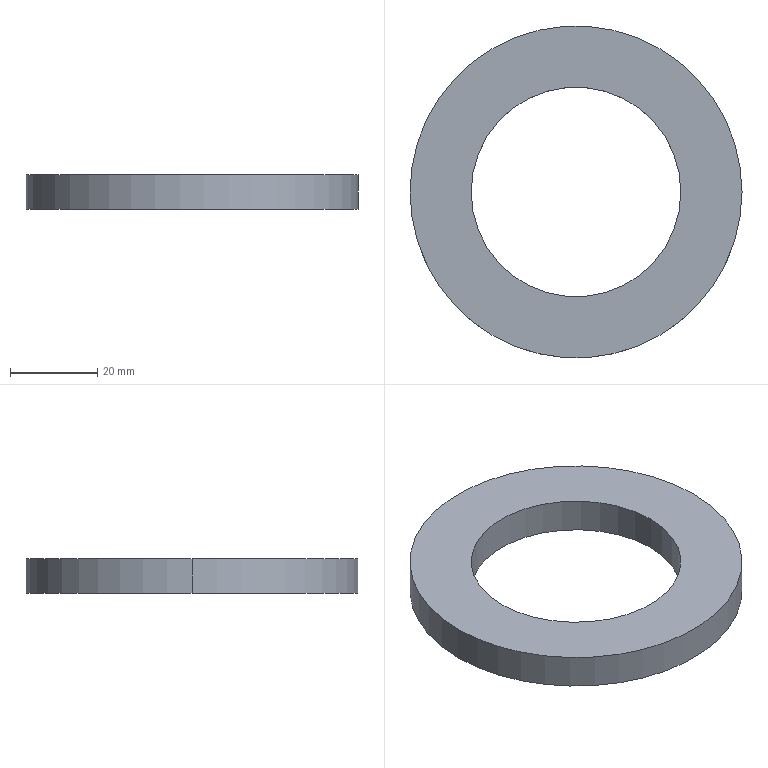Part | SolidWorks | features Extrusion 1 | 1 solid | 6 faces | box 76 x 76 x 8 mm | volume 21815 mm3 | cylinder 4 | plane 2 | commonest cylinder face diameters 48 x2 76 x2
STEP:
#1=CARTESIAN_POINT('',(-24.,0.,8.));
#2=VERTEX_POINT('',#1);
#3=CARTESIAN_POINT('',(24.,0.,8.));
#4=VERTEX_POINT('',#3);
#5=CARTESIAN_POINT('',(0.,0.,8.));
#6=DIRECTION('',(0.,0.,1.));
#7=DIRECTION('',(1.,0.,0.));
#8=AXIS2_PLACEMENT_3D('',#5,#6,#7);
#9=CIRCLE('',#8,24.);
#10=EDGE_CURVE('',#2,#4,#9,.T.);
#11=ORIENTED_EDGE('',*,*,#10,.T.);
#12=CARTESIAN_POINT('',(24.,0.,0.));
#13=VERTEX_POINT('',#12);
#14=CARTESIAN_POINT('',(24.,0.,8.));
#15=DIRECTION('',(0.,0.,-1.));
#16=VECTOR('',#15,1000.);
#17=LINE('',#14,#16);
#18=EDGE_CURVE('',#4,#13,#17,.T.);
#19=ORIENTED_EDGE('',*,*,#18,.T.);
#20=CARTESIAN_POINT('',(-24.,0.,0.));
#21=VERTEX_POINT('',#20);
#22=CARTESIAN_POINT('',(0.,0.,0.));
#23=DIRECTION('',(0.,0.,1.));
#24=DIRECTION('',(1.,0.,0.));
#25=AXIS2_PLACEMENT_3D('',#22,#23,#24);
#26=CIRCLE('',#25,24.);
#27=EDGE_CURVE('',#21,#13,#26,.T.);
#28=ORIENTED_EDGE('',*,*,#27,.F.);
#29=CARTESIAN_POINT('',(-24.,0.,8.));
#30=DIRECTION('',(0.,0.,-1.));
#31=VECTOR('',#30,1000.);
#32=LINE('',#29,#31);
#33=EDGE_CURVE('',#2,#21,#32,.T.);
#34=ORIENTED_EDGE('',*,*,#33,.F.);
#35=EDGE_LOOP('',(#11,#19,#28,#34));
#36=FACE_OUTER_BOUND('',#35,.T.);
#37=CARTESIAN_POINT('',(0.,0.,8.));
#38=DIRECTION('',(0.,0.,-1.));
#39=DIRECTION('',(-1.,0.,0.));
#40=AXIS2_PLACEMENT_3D('',#37,#38,#39);
#41=CYLINDRICAL_SURFACE('',#40,24.);
#42=ADVANCED_FACE('',(#36),#41,.F.);
#43=CARTESIAN_POINT('',(38.,0.,8.));
#44=VERTEX_POINT('',#43);
#45=CARTESIAN_POINT('',(-38.,0.,8.));
#46=VERTEX_POINT('',#45);
#47=CARTESIAN_POINT('',(0.,0.,8.));
#48=DIRECTION('',(0.,0.,1.));
#49=DIRECTION('',(1.,0.,0.));
#50=AXIS2_PLACEMENT_3D('',#47,#48,#49);
#51=CIRCLE('',#50,38.);
#52=EDGE_CURVE('',#44,#46,#51,.T.);
#53=ORIENTED_EDGE('',*,*,#52,.F.);
#54=CARTESIAN_POINT('',(38.,0.,0.));
#55=VERTEX_POINT('',#54);
#56=CARTESIAN_POINT('',(38.,0.,8.));
#57=DIRECTION('',(0.,0.,-1.));
#58=VECTOR('',#57,1000.);
#59=LINE('',#56,#58);
#60=EDGE_CURVE('',#44,#55,#59,.T.);
#61=ORIENTED_EDGE('',*,*,#60,.T.);
#62=CARTESIAN_POINT('',(-38.,0.,0.));
#63=VERTEX_POINT('',#62);
#64=CARTESIAN_POINT('',(0.,0.,0.));
#65=DIRECTION('',(0.,0.,1.));
#66=DIRECTION('',(1.,0.,0.));
#67=AXIS2_PLACEMENT_3D('',#64,#65,#66);
#68=CIRCLE('',#67,38.);
#69=EDGE_CURVE('',#55,#63,#68,.T.);
#70=ORIENTED_EDGE('',*,*,#69,.T.);
#71=CARTESIAN_POINT('',(-38.,0.,8.));
#72=DIRECTION('',(0.,0.,-1.));
#73=VECTOR('',#72,1000.);
#74=LINE('',#71,#73);
#75=EDGE_CURVE('',#46,#63,#74,.T.);
#76=ORIENTED_EDGE('',*,*,#75,.F.);
#77=EDGE_LOOP('',(#53,#61,#70,#76));
#78=FACE_OUTER_BOUND('',#77,.T.);
#79=CARTESIAN_POINT('',(0.,0.,8.));
#80=DIRECTION('',(0.,0.,-1.));
#81=DIRECTION('',(-1.,0.,0.));
#82=AXIS2_PLACEMENT_3D('',#79,#80,#81);
#83=CYLINDRICAL_SURFACE('',#82,38.);
#84=ADVANCED_FACE('',(#78),#83,.T.);
#85=CARTESIAN_POINT('',(0.,0.,8.));
#86=DIRECTION('',(0.,0.,1.));
#87=DIRECTION('',(1.,0.,0.));
#88=AXIS2_PLACEMENT_3D('',#85,#86,#87);
#89=CIRCLE('',#88,38.);
#90=EDGE_CURVE('',#46,#44,#89,.T.);
#91=ORIENTED_EDGE('',*,*,#90,.T.);
#92=ORIENTED_EDGE('',*,*,#52,.T.);
#93=EDGE_LOOP('',(#91,#92));
#94=FACE_OUTER_BOUND('',#93,.T.);
#95=ORIENTED_EDGE('',*,*,#10,.F.);
#96=CARTESIAN_POINT('',(0.,0.,8.));
#97=DIRECTION('',(0.,0.,1.));
#98=DIRECTION('',(1.,0.,0.));
#99=AXIS2_PLACEMENT_3D('',#96,#97,#98);
#100=CIRCLE('',#99,24.);
#101=EDGE_CURVE('',#4,#2,#100,.T.);
#102=ORIENTED_EDGE('',*,*,#101,.F.);
#103=EDGE_LOOP('',(#95,#102));
#104=FACE_BOUND('',#103,.T.);
#105=CARTESIAN_POINT('',(0.,0.,8.));
#106=DIRECTION('',(0.,0.,1.));
#107=DIRECTION('',(1.,0.,0.));
#108=AXIS2_PLACEMENT_3D('',#105,#106,#107);
#109=PLANE('',#108);
#110=ADVANCED_FACE('',(#94,#104),#109,.T.);
#111=CARTESIAN_POINT('',(0.,0.,0.));
#112=DIRECTION('',(0.,0.,1.));
#113=DIRECTION('',(1.,0.,0.));
#114=AXIS2_PLACEMENT_3D('',#111,#112,#113);
#115=CIRCLE('',#114,38.);
#116=EDGE_CURVE('',#63,#55,#115,.T.);
#117=ORIENTED_EDGE('',*,*,#116,.F.);
#118=ORIENTED_EDGE('',*,*,#69,.F.);
#119=EDGE_LOOP('',(#117,#118));
#120=FACE_OUTER_BOUND('',#119,.T.);
#121=ORIENTED_EDGE('',*,*,#27,.T.);
#122=CARTESIAN_POINT('',(0.,0.,0.));
#123=DIRECTION('',(0.,0.,1.));
#124=DIRECTION('',(1.,0.,0.));
#125=AXIS2_PLACEMENT_3D('',#122,#123,#124);
#126=CIRCLE('',#125,24.);
#127=EDGE_CURVE('',#13,#21,#126,.T.);
#128=ORIENTED_EDGE('',*,*,#127,.T.);
#129=EDGE_LOOP('',(#121,#128));
#130=FACE_BOUND('',#129,.T.);
#131=CARTESIAN_POINT('',(0.,0.,0.));
#132=DIRECTION('',(0.,0.,1.));
#133=DIRECTION('',(1.,0.,0.));
#134=AXIS2_PLACEMENT_3D('',#131,#132,#133);
#135=PLANE('',#134);
#136=ADVANCED_FACE('',(#120,#130),#135,.F.);
#137=ORIENTED_EDGE('',*,*,#60,.F.);
#138=ORIENTED_EDGE('',*,*,#90,.F.);
#139=ORIENTED_EDGE('',*,*,#75,.T.);
#140=ORIENTED_EDGE('',*,*,#116,.T.);
#141=EDGE_LOOP('',(#137,#138,#139,#140));
#142=FACE_OUTER_BOUND('',#141,.T.);
#143=CARTESIAN_POINT('',(0.,0.,8.));
#144=DIRECTION('',(0.,0.,-1.));
#145=DIRECTION('',(-1.,0.,0.));
#146=AXIS2_PLACEMENT_3D('',#143,#144,#145);
#147=CYLINDRICAL_SURFACE('',#146,38.);
#148=ADVANCED_FACE('',(#142),#147,.T.);
#149=ORIENTED_EDGE('',*,*,#18,.F.);
#150=ORIENTED_EDGE('',*,*,#101,.T.);
#151=ORIENTED_EDGE('',*,*,#33,.T.);
#152=ORIENTED_EDGE('',*,*,#127,.F.);
#153=EDGE_LOOP('',(#149,#150,#151,#152));
#154=FACE_OUTER_BOUND('',#153,.T.);
#155=CARTESIAN_POINT('',(0.,0.,8.));
#156=DIRECTION('',(0.,0.,-1.));
#157=DIRECTION('',(-1.,0.,0.));
#158=AXIS2_PLACEMENT_3D('',#155,#156,#157);
#159=CYLINDRICAL_SURFACE('',#158,24.);
#160=ADVANCED_FACE('',(#154),#159,.F.);
#161=CLOSED_SHELL('',(#42,#84,#110,#136,#148,#160));
#162=MANIFOLD_SOLID_BREP('',#161);
#163=CARTESIAN_POINT('',(0.,0.,0.));
#164=DIRECTION('',(0.,0.,1.));
#165=DIRECTION('',(1.,0.,0.));
#166=AXIS2_PLACEMENT_3D('',#163,#164,#165);
#167=(LENGTH_UNIT()NAMED_UNIT(*)SI_UNIT(.MILLI.,.METRE.));
#168=UNCERTAINTY_MEASURE_WITH_UNIT(LENGTH_MEASURE(0.00001),#167,'','');
#169=(NAMED_UNIT(*)PLANE_ANGLE_UNIT()SI_UNIT($,.RADIAN.));
#170=(NAMED_UNIT(*)SI_UNIT($,.STERADIAN.)SOLID_ANGLE_UNIT());
#171=(GEOMETRIC_REPRESENTATION_CONTEXT(3)GLOBAL_UNCERTAINTY_ASSIGNED_CONTEXT((#168))GLOBAL_UNIT_ASSIGNED_CONTEXT((#167,#169,#170))REPRESENTATION_CONTEXT('',''));
#172=ADVANCED_BREP_SHAPE_REPRESENTATION('',(#162,#166),#171);